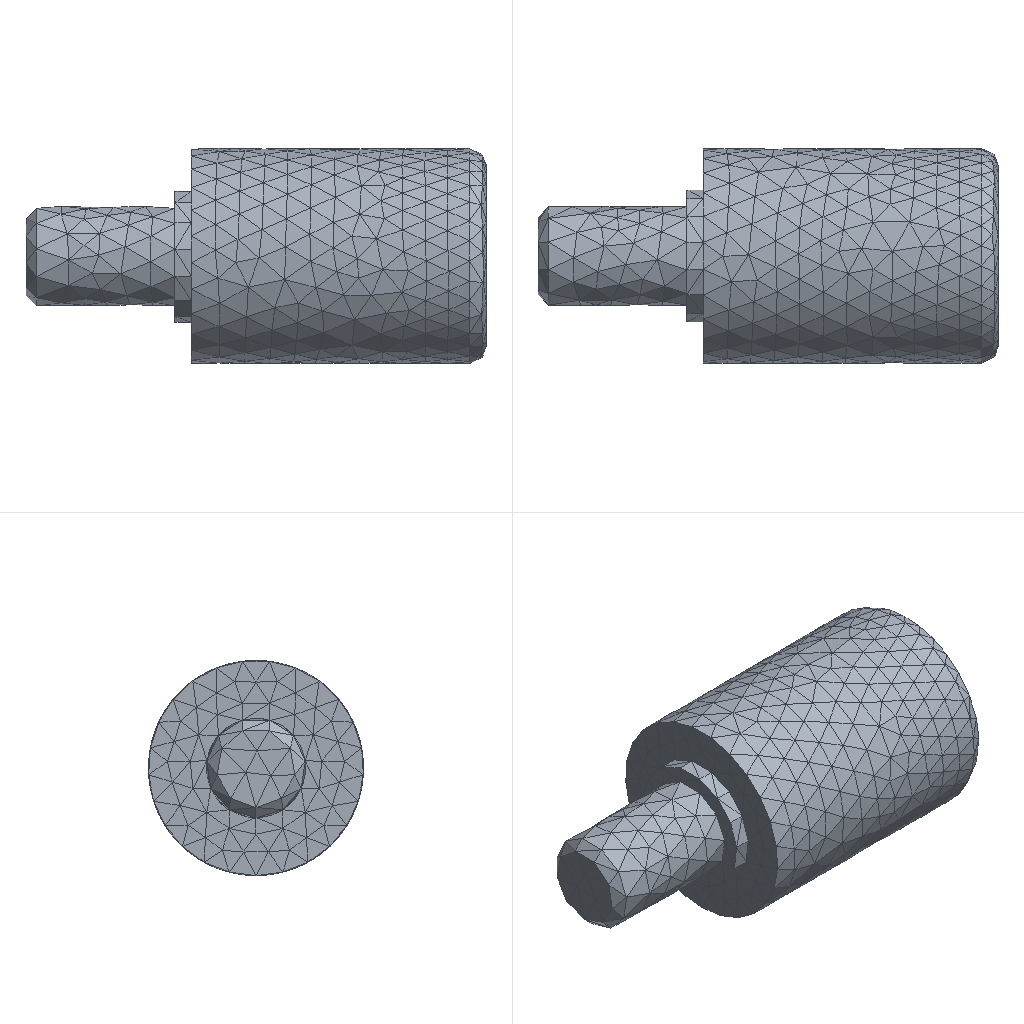Simulation study | ansys workbench
Set-up summary:
category,name,step,type,value,unit,region
solver,ansys_mapdl
solver,version,,,25.2
units,MPA,,stated
analysis,deck,,static,static
load_step,requested,,,1
analysis,nlgeom,,,False
mesh,nodes,,,6848
mesh,elements,,,5381
element_type,ANSYS 291 (type 1),,thermal_solid,4168
element_type,ANSYS 152 (type 2),,surface,1213
load,load commands in deck,,count,3
bc,support commands in deck,,count,2
named_set,_CM31,,component
named_set,_ELMISC,,component
material,1,,in results
check,setup vs results,,match,1213 surface effect element(s) are not in the reader's mesh and were not compared
Ansys APDL input file, long lists of numbers shortened:
/batch
/config,noeldb,1     ! force off writing results to database
*get,_wallstrt,active,,time,wall
! ANSYS input file written by Workbench version 2025 R2
! File used for geometry attach: C:\Users\lenovo\Desktop\CAE\1317\1317.x_t
/title,wbnew--___ (A5)
! ****** Begin Custom Load Command Snippet ******
/COM, ACT Extensions:
/COM,     LSDYNA, 2025.2
/COM,/COM,     ANSYSMotion, 2025.2
/COM,
! ****** End   Custom Load Command Snippet ******
*DIM,_wb_ProjectScratch_dir,string,248
_wb_ProjectScratch_dir(1) = 'C:\Users\lenovo\AppData\Local\Temp\WB_lenovo_13032_2\_ProjectScratch\Scr43A9\'
*DIM,_wb_SolverFiles_dir,string,248
_wb_SolverFiles_dir(1) = 'C:\Users\lenovo\AppData\Local\Temp\WB_lenovo_13032_2\wbnew_files\dp0\SYS\MECH\'
*DIM,_wb_userfiles_dir,string,248
_wb_userfiles_dir(1) = 'C:\Users\lenovo\AppData\Local\Temp\WB_lenovo_13032_2\wbnew_files\user_files\'
/com,--- Data in consistent NMM units. See Solving Units in the help system for more information.
/units,MPA
/nopr
/wb,file,start              !  signify a WB generated input file
/prep7
! Turn off shape checking because checks already performed inside WB mesher.
! See help system for more information.
SHPP,OFF,,NOWARN
/nolist
etcon,set             ! allow ANSYS to choose best KEYOP's for 180x elements, resets any applicable keyopt to MAPDL defaults
/com,*********** Send User Defined Coordinate System(s) ***********
csys,0
/com,*********** Nodes for the whole assembly ***********
nblock,3,,7532
(1i9,3e20.9e3)
        1     1.830000000E+01    -3.867815921E+00     5.000000000E-01
! (6847 more lines like these left out)
-1
/wb,elem,start            !  set before creation of elements
/com,*********** Elements for Body 1 'Part 1' ***********
et,1,291
MAT,1 $ TYPE,1 $ REAL,1 $ SECNUM,1 $ ESYS,0
eblock,11,COMPACT,,4168
(11i9)
        1      982      984     1034     1013     6761     6773     6765     6764     6769     6834
! (4167 more lines like these left out)
-1
secnum,1    ! reset the section ID to default
/wb,elem,end               !  done creating elements
toffst,273.15,      ! Temperature offset from absolute zero
/wb,mat,start              !  starting to send materials
/com,*********** Send Materials ***********
Temperature = 'TEMP' ! Temperature
MP,KXX,1,237,	! tonne mm s^-3 C^-1
/wb,mat,end                !  done sending materials
!************************* Model Summary ********************
!Part 1,	01,	matid,	1
!************************* End Model Summary ********************
! get the diagonal of the bounding box. Needed later for other things
*get,_xmin,node,,mnloc,x
*get,_ymin,node,,mnloc,y
*get,_zmin,node,,mnloc,z
*get,_xmax,node,,mxloc,x
*get,_ymax,node,,mxloc,y
*get,_zmax,node,,mxloc,z
_ASMDIAG=(_xmax-_xmin)*(_xmax-_xmin)+(_ymax-_ymin)*(_ymax-_ymin)+(_zmax-_zmin)*(_zmax-_zmin)
_ASMDIAG=SQRT(_ASMDIAG)
/wb,contact,start          !  starting to send contact
/wb,contact,end            !  done creating contacts
/golist
/wb,load,start             !  starting to send loads
/com,*********** Define Temperature Constraint ***********
CMBLOCK,_CM31   ,NODE,       28
(8i10)
        13       -21       607      -609      1145      1146      1150      1151
      1153      1156      1159      1162      1164      1167      1168      1171
      1174      1177      1181      1185      1188      1189      1191      1194
      1199      4726      4727      4732
fcum,add                   ! add nodal forces up (needed in case have loads on the same edge,vertex)
fcum                       ! reset default on fcum command since done sending WB F loads
/com,*********** Create "______" ***********
et,2,152
MAT,2 $ TYPE,2 $ REAL,2 $ SECNUM,2 $ ESYS,0
eblock,11,COMPACT,,1213
(11i9)
     5395        7      614        8        8     1106     1117        8     1102
! (1212 more lines like these left out)
-1
secnum,1    ! reset the section ID to default
esel,s,type,,2
keyop,2,8,2
keyop,2,13,0
esel,all
/com,***************** Define Uniform Initial temperature ***************
tunif,22.
/gst,on,on
fini
*get,_numnode,node,0,count
*get,_numelem,elem,0,count
*get, _MAXELEMNUM, elem, 0, NUM, MAX
*get, _MAXNODENUM, node, 0, NUM, MAX
*get, _MAXELEMTYPE, etyp, 0, NUM, MAX
*get, _MAXREALCONST, rcon, 0, NUM, MAX
/go
/wb,load,end               !  done creating loads
/com,--- Number of total nodes = %_numnode%
/com,--- Number of contact elements = 1213
/com,--- Number of spring elements = 0
/com,--- Number of bearing elements = 0
/com,--- Number of solid elements = 4168
/com,--- Number of condensed parts = 0
/com,--- Number of total elements = %_numelem%
*get,_wallbsol,active,,time,wall
/com,****************************************************************************
/com,*************************    SOLUTION       ********************************
/com,****************************************************************************
/solu
antype,0                   ! static analysis
!eqsl,sparse               ! using sparse solver which is default so no eqsl command needed
cntr,print,1               ! print out contact info and also make no initial contact an error
cncheck,dmp		!	Enable program controlled contact splitting for distributed memory parallel run
rescontrol,,none                 ! Do not keep any restart files
dmpoption,emat,no             ! Don't combine emat file for DANSYS
dmpoption,esav,no             ! Don't combine esav file for DANSYS
/com,****************************************************
/com,******************* SOLVE FOR LS 1 OF 1 ****************
d,_CM31,temp,500.
esel,s,type,,2
nsle
sf,all,conv,0.237,25.
nsel,all
esel,all
/nopr
/gopr
autots,on
nsub,1,10,1
time,1.
outres,erase
outres,all,none
outres,nsol,all
outres,rsol,all
outres,eangl,all
outres,veng,all
outres,fflux,all,
outres,cont,all,
/nopr
esel,s,type,,2
cm,_elmisc,elem
esel,all
/gopr
outres,misc,all,_elmisc
cnvtol,heat,,1.e-003,,1.e-003 ! Program Controlled. Set MINREF equivalent of 1e-6 Watts
! *********** WB SOLVE COMMAND ***********
! check interactive state
*get,ANSINTER_,active,,int
*if,ANSINTER_,ne,0,then
/eof
*endif
solve
/com *************** Write FE CONNECTORS *********
CEWRITE,file,ce,,INTE
/com,****************************************************
/com,*************** FINISHED SOLVE FOR LS 1 *************
*get,_wallasol,active,,time,wall
/post1
xmlo,ENCODING,ISO-8859-1
xmlo,parm
/xml,parm,xml
fini
/gopr
*get,_walldone,active,,time,wall
_preptime=(_wallbsol-_wallstrt)*3600
_solvtime=(_wallasol-_wallbsol)*3600
_posttime=(_walldone-_wallasol)*3600
_totaltim=(_walldone-_wallstrt)*3600
*get,_dlbratio,active,0,solu,dlbr
*get,_combtime,active,0,solu,comb
*get,_ssmode,active,0,solu,ssmm
*get,_ndofs,active,0,solu,ndof
/fclean				!clean distributed files
/com,--- Total number of nodes = %_numnode%
/com,--- Total number of elements = %_numelem%
/com,--- Element load balance ratio = %_dlbratio%
/com,--- Time to combine distributed files = %_combtime%
/com,--- Sparse memory mode = %_ssmode%
/com,--- Number of DOF = %_ndofs%
/wb,file,end               ! done with WB generated input
Results summary:
result,analysis,,,static
result,last_loadstep,,,1
result,primary field,,,temperature